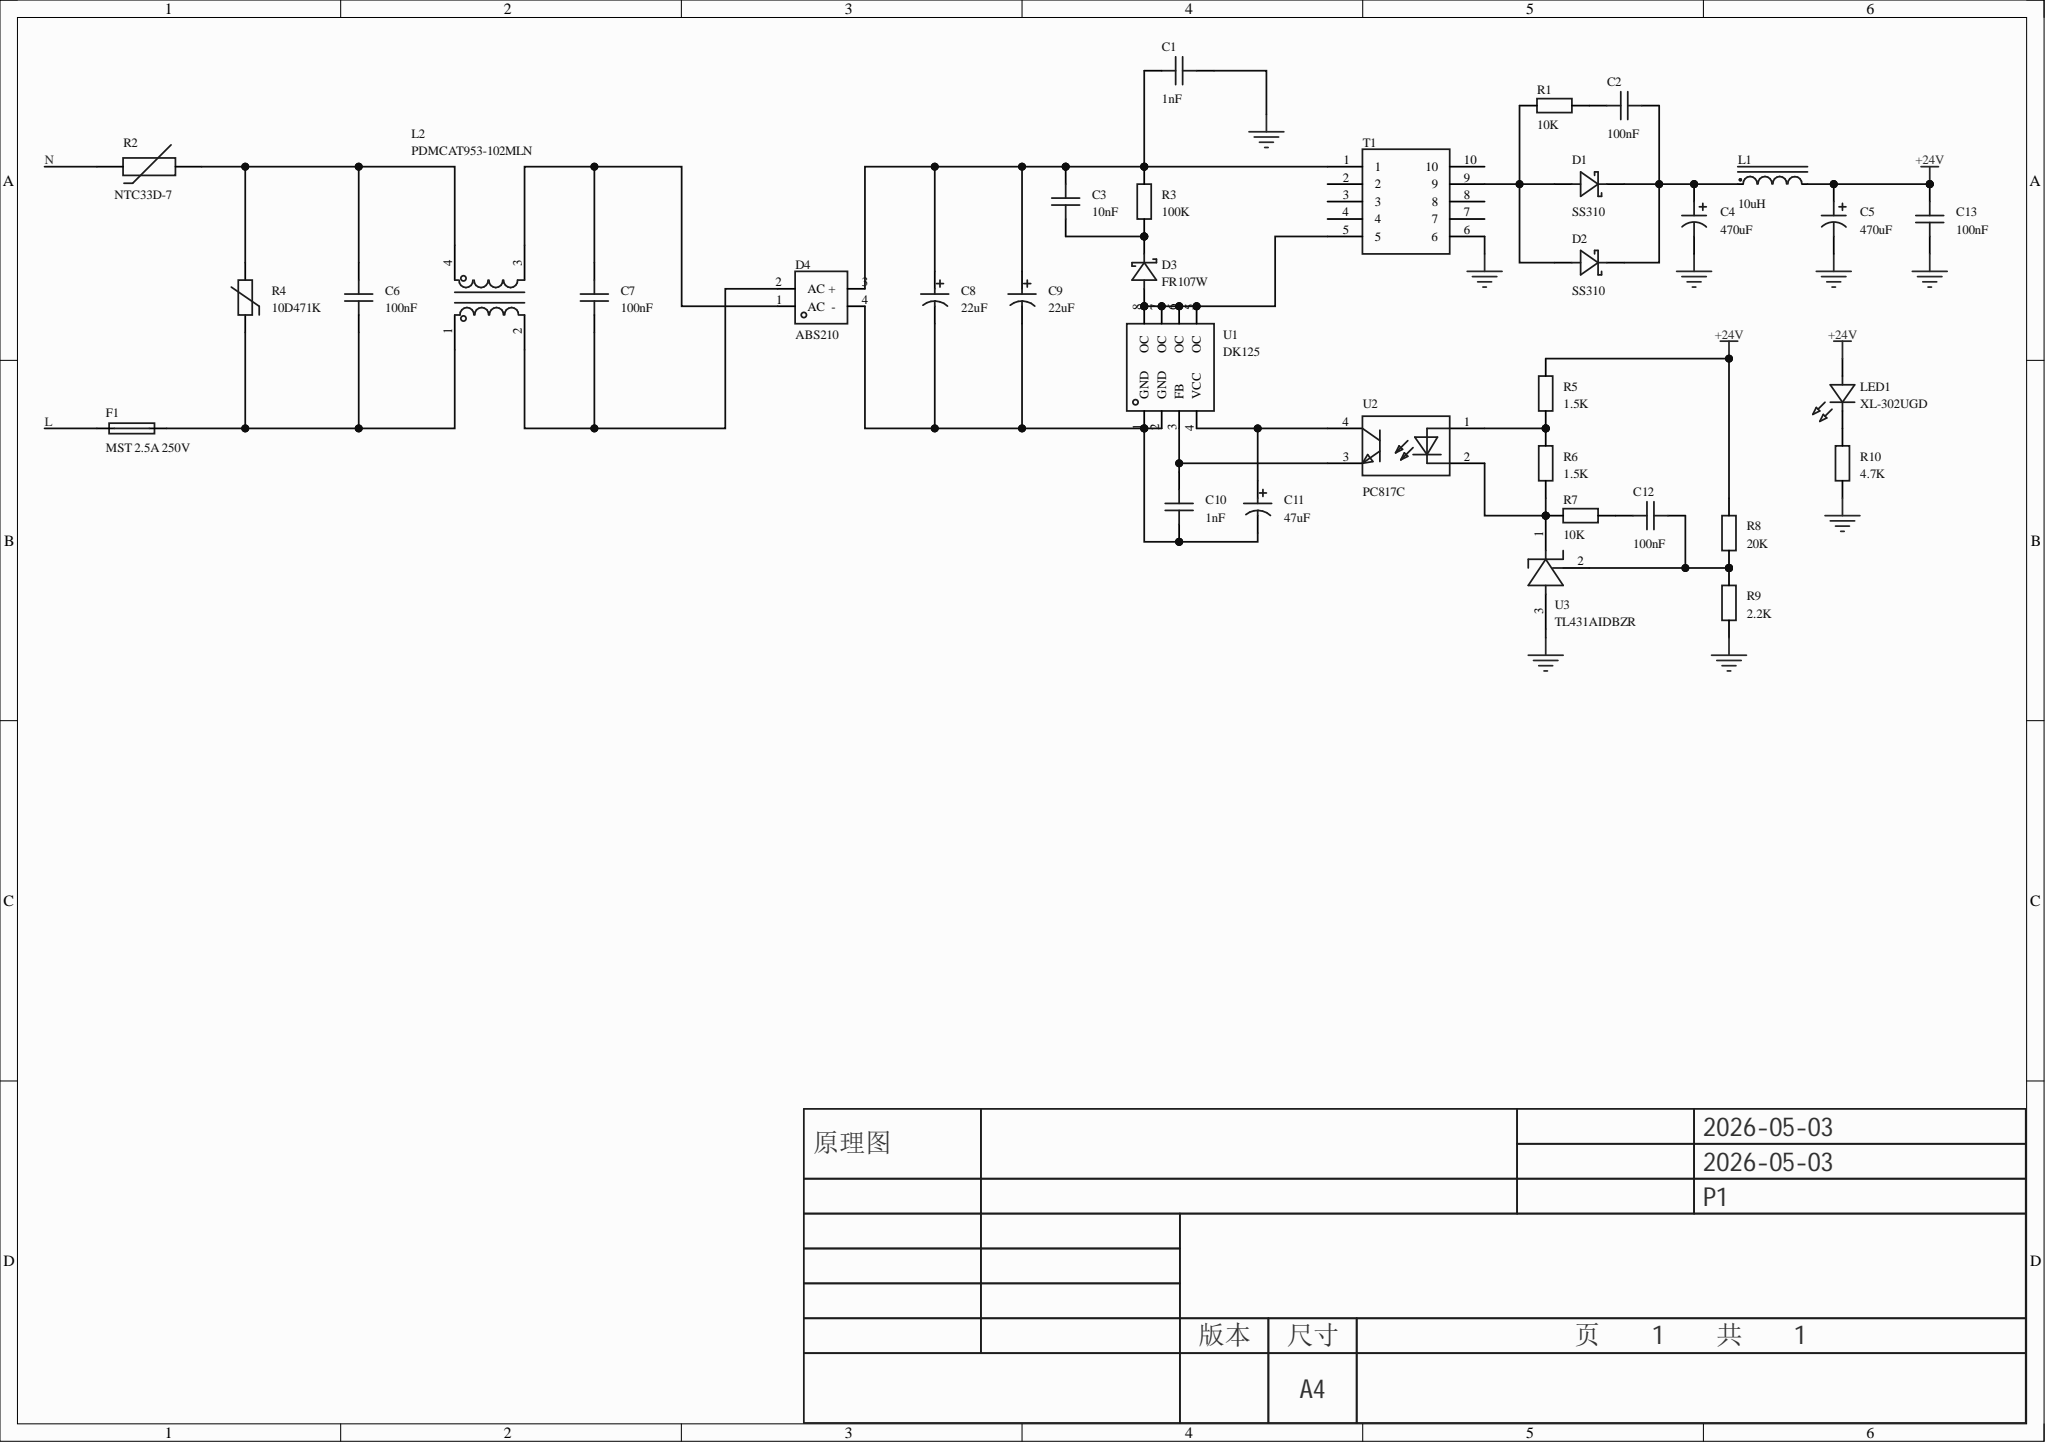Circuit board | Altium Designer | 35 parts | 20 nets
Bill of materials:
Comment,Description,Designator,Footprint,LibRef,Quantity
"1nF","容值:1nF;精度:±20%;工作电压(AC):400V;防护等级:Y1;","C1","CAP-TH_L7.5-W4.5-P10.00-D0.6","KY1102M400VAC70Y10093","1"
"100nF","","C2, C12, C13","C0603","CAP_0603","3"
"10nF","","C3","C1206","CAP_0603","1"
"470uF","","C4, C5","CAP-TH_BD8.0-P3.50-D0.6-FD","JBLH2471M035D140RLM 470UF 35V","2"
"100nF","容值:100nF;精度:±10%;工作电压(AC):275V；310V；305V;防护等级:X2;","C6, C7","CAP-TH_L13.0-W6.0-P10.00-D0.6","MPX104K31C3KN15600","2"
"22uF","容值:22uF;精度:±20%;额定电压:400V;纹波电流:-;等效串联电阻(ESR):-;","C8, C9","CAP-TH_BD10.0-P5.00-D1.0-FD","ERK2GM220G16OT","2"
"1nF","","C10","C0603","CAP_0603","1"
"47uF","容值:47uF;精度:±20%;额定电压:25V;","C11","CAP-TH_BD5.0-P2.00-D0.8-FD","KS476M025D07RR0VH2FP0","1"
"SS310","二极管配置:独立式;正向压降(Vf):850mV@3A;直流反向耐压(Vr):100V;整流电流:3A;","D1, D2","SMA_L4.3-W2.6-LS5.0-FD","SS310_C7420364","2"
"FR107W","二极管配置:独立式;正向压降(Vf):1.3V@1.0A;直流反向耐压(Vr):1kV;整流电流:1A;反向恢复时间(Trr):500ns;","D3","SOD-123FL_L2.7-W1.8-LS3.8-RD","FR107W_C18199114","1"
"ABS210","正向压降(Vf):1V@1A;直流反向耐压(Vr):1kV;整流电流:2A;非重复峰值浪涌电流 (Ifsm):60A;","D4","ABF_L5.1-W4.4-P4.00-LS6.2-BL","ABS210_C42406052","1"
"MST 2.5A 250V","类型:-;额定电流:2.5A;","F1","FUSE-TH_L8.4-W4.3-P5.08-D1.0","MST 2.5A 250V","1"
"10uH","电感值:10uH;精度:±10%;类型:工字电感;","L1","IND-TH_BD8.0-P5.00-D0.7","XR8*10-100K-L","1"
"PDMCAT953-102MLN","","L2","IND-TH_4P-L12.0-W6.0_PDMCAT953-501MLN","PDMCAT953-102MLN","1"
"XL-302UGD","灯头类型:3mm圆形灯头;发光颜色:翠绿色;正向压降(Vf):3.6V;功率:70mW;正向电流:20mA;波长:520nm~530nm;透镜颜色:绿色透镜;色温:-;发光强度:3000mcd;发光角度:30°;载带方式:-;工作温度:-20℃~+85℃;","LED1","LED-TH_BD3.8-P2.54-FD_GREEN","XL-302UGD","1"
"10K","","R1, R7","R0603","Res_0603","2"
"NTC33D-7","","R2","RES-TH_L6.5-W5.0-P5.00-D0.6-S4.40","NTC33D-7","1"
"100K","","R3","R1206","Res_0603","1"
"10D471K","压敏电压:470V;钳位电压:775V;工作电压(DC):385V;工作电压(AC):300V;","R4","RES-TH_L11.0-W6.0-P7.50-D0.8-S3.00","10D471K_C49072849","1"
"1.5K","","R5, R6","R0603","Res_0603","2"
"20K","","R8","R0603","Res_0603","1"
"2.2K","","R9","R0603","Res_0603","1"
"4.7K","","R10","R0603","Res_0603","1"
"","","T1","EE25 5+5","EE25","1"
"DK125","工作电压:4.5V~4.9V;开关频率:61kHz~69kHz;晶体管耐压:700V;","U1","DIP-8_L9.2-W6.4-P2.54-LS7.6-BL","DK125","1"
"PC817C","输入类型:DC;正向压降(Vf):1.2V;输出电流:50mA;隔离电压(Vrms):5kV;直流反向耐压(Vr):6V;负载电压:35V;输出通道数:1;集射极饱和电压(VCE(sat)):100mV@1mA,20mA;","U2","DIP-4_L4.6-W6.5-P2.54-LS7.6-BL","PC817C_C3025068","1"
"TL431AIDBZR","输出类型:可调;输入电压:-;输出电压:2.495V~36V;输出电流:100mA;精度:±1%;","U3","SOT-23-3_L2.9-W1.6-P1.90-LS2.8-BR","TL431AIDBZR","1"
Netlist (Protel format):
[
C1
CAP-TH_L7.5-W4.5-P10.00-D0.6
1nF



]
[
C2
C0603
100nF



]
[
C3
C1206
10nF



]
[
C4
CAP-TH_BD8.0-P3.50-D0.6-FD
470uF



]
[
C5
CAP-TH_BD8.0-P3.50-D0.6-FD
470uF



]
[
C6
CAP-TH_L13.0-W6.0-P10.00-D0.6
100nF



]
[
C7
CAP-TH_L13.0-W6.0-P10.00-D0.6
100nF



]
[
C8
CAP-TH_BD10.0-P5.00-D1.0-FD
22uF



]
[
C9
CAP-TH_BD10.0-P5.00-D1.0-FD
22uF



]
[
C10
C0603
1nF



]
[
C11
CAP-TH_BD5.0-P2.00-D0.8-FD
47uF



]
[
C12
C0603
100nF



]
[
C13
C0603
100nF



]
[
D1
SMA_L4.3-W2.6-LS5.0-FD
SS310



]
[
D2
SMA_L4.3-W2.6-LS5.0-FD
SS310



]
[
D3
SOD-123FL_L2.7-W1.8-LS3.8-RD
FR107W



]
[
D4
ABF_L5.1-W4.4-P4.00-LS6.2-BL
ABS210



]
[
F1
FUSE-TH_L8.4-W4.3-P5.08-D1.0
MST 2.5A 250V



]
[
L1
IND-TH_BD8.0-P5.00-D0.7
10uH



]
[
L2
IND-TH_4P-L12.0-W6.0_PDMCAT953-501MLN
PDMCAT953-102MLN



]
[
LED1
LED-TH_BD3.8-P2.54-FD_GREEN
XL-302UGD



]
[
R1
R0603
10K



]
[
R2
RES-TH_L6.5-W5.0-P5.00-D0.6-S4.40
NTC33D-7



]
[
R3
R1206
100K



]
[
R4
RES-TH_L11.0-W6.0-P7.50-D0.8-S3.00
10D471K



]
[
R5
R0603
1.5K



]
[
R6
R0603
1.5K



]
[
R7
R0603
10K



]
[
R8
R0603
20K



]
[
R9
R0603
2.2K



]
[
R10
R0603
4.7K



]
[
T1
EE25 5+5




]
[
U1
DIP-8_L9.2-W6.4-P2.54-LS7.6-BL
DK125



]
[
U2
DIP-4_L4.6-W6.5-P2.54-LS7.6-BL
PC817C



]
[
U3
SOT-23-3_L2.9-W1.6-P1.90-LS2.8-BR
TL431AIDBZR



]
(
NetR6_1
R6-1
R7-1
U2-2
U3-1
)
(
NetR5_1
R5-1
R6-2
U2-1
)
(
NetLED1_2
LED1-2
R10-2
)
(
NetD3_2
D3-2
T1-5
U1-5
U1-6
U1-7
U1-8
)
(
NetD1_1
D1-1
D2-1
R1-1
T1-9
)
(
NetC12_2
C12-2
R7-2
)
(
NetC12_1
C12-1
R8-1
R9-2
U3-2
)
(
NetC11_1
C11-1
U1-4
U2-4
)
(
NetC10_2
C10-2
U1-3
U2-3
)
(
NetC8_2
C8-2
C9-2
C10-1
C11-2
D4-4
U1-1
U1-2
)
(
NetC7_2
C7-2
D4-2
L2-2
)
(
NetC7_1
C7-1
D4-1
L2-3
)
(
NetC6_2
C6-2
F1-2
L2-1
R4-1
)
(
NetC6_1
C6-1
L2-4
R2-2
R4-2
)
(
NetC3_1
C3-1
D3-1
R3-1
)
(
NetC2_2
C2-2
C4-1
D1-2
D2-2
L1-1
)
(
NetC2_1
C2-1
R1-2
)
(
NetC1_1
C1-1
C3-2
C8-1
C9-1
D4-3
R3-2
T1-1
)
(
GND
C1-2
C4-2
C5-2
C13-1
R9-1
R10-1
T1-6
U3-3
)
(
+24V
C5-1
C13-2
L1-2
LED1-1
R5-2
R8-2
)